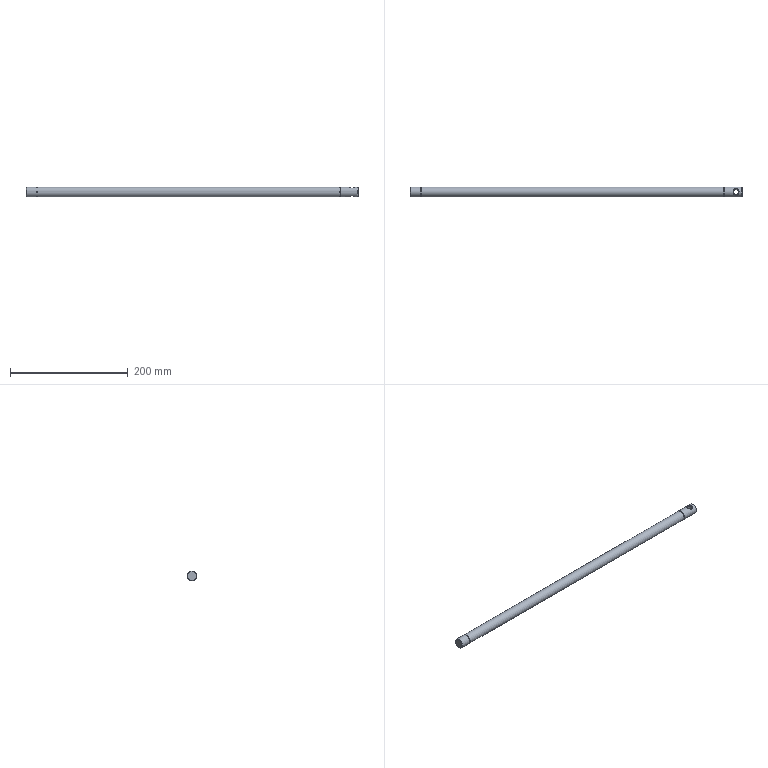Part | STEP file | 610B0702 | 1 solid | 16 faces | box 565 x 17 x 17 mm | volume 128554 mm3 | plane 6 | cylinder 6 | cone 2 | spline 2 | commonest cylinder face diameters 17 x3 15 x2 8 x1